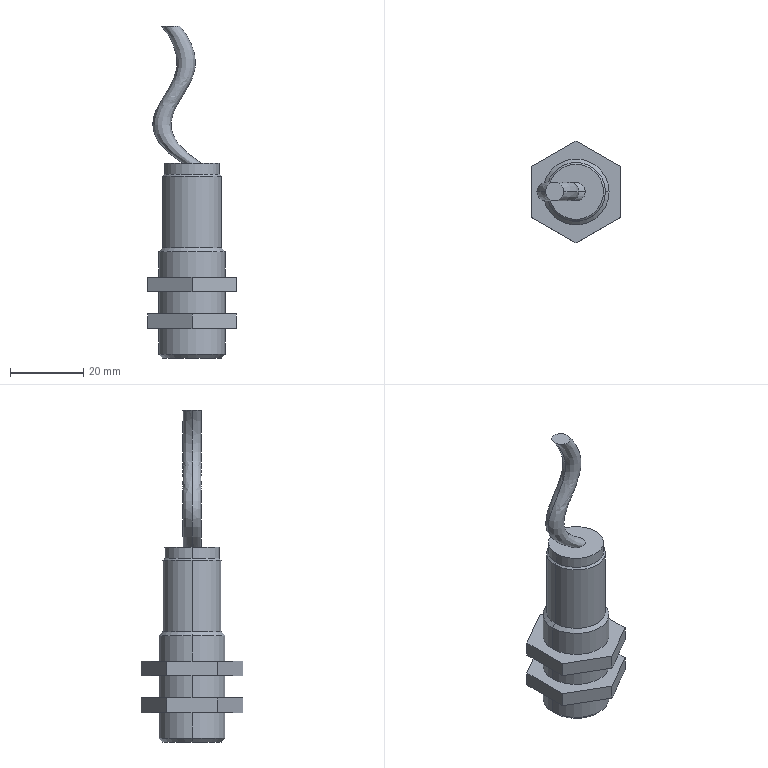Part | SolidWorks | features ICE 3, Chamfer 2, Extrusion 1, MirrorPattern 1, Sweep 1 | 1 solid | 37 faces | box 24 x 27.713 x 90.43 mm | volume 14815 mm3 | plane 19 | cylinder 10 | cone 6 | spline 2 | commonest cylinder face diameters 18 x6 15 x2 16 x2
STEP:
#1=CARTESIAN_POINT('',(9.,0.,-7.));
#2=VERTEX_POINT('',#1);
#3=CARTESIAN_POINT('',(-9.,0.,-7.));
#4=VERTEX_POINT('',#3);
#5=CARTESIAN_POINT('',(0.,0.,-7.));
#6=DIRECTION('',(0.,0.,1.));
#7=DIRECTION('',(1.,0.,0.));
#8=AXIS2_PLACEMENT_3D('',#5,#6,#7);
#9=CIRCLE('',#8,9.);
#10=EDGE_CURVE('',#2,#4,#9,.T.);
#11=ORIENTED_EDGE('',*,*,#10,.F.);
#12=CARTESIAN_POINT('',(9.,0.,-14.));
#13=VERTEX_POINT('',#12);
#14=CARTESIAN_POINT('',(9.,0.,15.));
#15=DIRECTION('',(0.,0.,-1.));
#16=VECTOR('',#15,1000.);
#17=LINE('',#14,#16);
#18=EDGE_CURVE('',#2,#13,#17,.T.);
#19=ORIENTED_EDGE('',*,*,#18,.T.);
#20=CARTESIAN_POINT('',(-9.,0.,-14.));
#21=VERTEX_POINT('',#20);
#22=CARTESIAN_POINT('',(0.,0.,-14.));
#23=DIRECTION('',(0.,0.,1.));
#24=DIRECTION('',(1.,0.,0.));
#25=AXIS2_PLACEMENT_3D('',#22,#23,#24);
#26=CIRCLE('',#25,9.);
#27=EDGE_CURVE('',#13,#21,#26,.T.);
#28=ORIENTED_EDGE('',*,*,#27,.T.);
#29=CARTESIAN_POINT('',(-9.,0.,15.));
#30=DIRECTION('',(0.,0.,-1.));
#31=VECTOR('',#30,1000.);
#32=LINE('',#29,#31);
#33=EDGE_CURVE('',#4,#21,#32,.T.);
#34=ORIENTED_EDGE('',*,*,#33,.F.);
#35=EDGE_LOOP('',(#11,#19,#28,#34));
#36=FACE_OUTER_BOUND('',#35,.T.);
#37=CARTESIAN_POINT('',(0.,0.,15.));
#38=DIRECTION('',(0.,0.,-1.));
#39=DIRECTION('',(-1.,0.,0.));
#40=AXIS2_PLACEMENT_3D('',#37,#38,#39);
#41=CYLINDRICAL_SURFACE('',#40,9.);
#42=ADVANCED_FACE('',(#36),#41,.T.);
#43=CARTESIAN_POINT('',(-8.,0.,-15.));
#44=VERTEX_POINT('',#43);
#45=CARTESIAN_POINT('',(8.,0.,-15.));
#46=VERTEX_POINT('',#45);
#47=CARTESIAN_POINT('',(0.,0.,-15.));
#48=DIRECTION('',(0.,0.,-1.));
#49=DIRECTION('',(1.,0.,0.));
#50=AXIS2_PLACEMENT_3D('',#47,#48,#49);
#51=CIRCLE('',#50,8.);
#52=EDGE_CURVE('',#44,#46,#51,.T.);
#53=ORIENTED_EDGE('',*,*,#52,.F.);
#54=CARTESIAN_POINT('',(-9.,0.,-14.));
#55=DIRECTION('',(-0.7071,0.,0.7071));
#56=VECTOR('',#55,1000.);
#57=LINE('',#54,#56);
#58=EDGE_CURVE('',#44,#21,#57,.T.);
#59=ORIENTED_EDGE('',*,*,#58,.T.);
#60=ORIENTED_EDGE('',*,*,#27,.F.);
#61=CARTESIAN_POINT('',(9.,0.,-14.));
#62=DIRECTION('',(0.7071,0.,0.7071));
#63=VECTOR('',#62,1000.);
#64=LINE('',#61,#63);
#65=EDGE_CURVE('',#46,#13,#64,.T.);
#66=ORIENTED_EDGE('',*,*,#65,.F.);
#67=EDGE_LOOP('',(#53,#59,#60,#66));
#68=FACE_OUTER_BOUND('',#67,.T.);
#69=CARTESIAN_POINT('',(0.,0.,-14.));
#70=DIRECTION('',(0.,0.,1.));
#71=DIRECTION('',(1.,0.,0.));
#72=AXIS2_PLACEMENT_3D('',#69,#70,#71);
#73=CONICAL_SURFACE('',#72,9.,0.7854);
#74=ADVANCED_FACE('',(#68),#73,.T.);
#75=CARTESIAN_POINT('',(2.5,0.,38.));
#76=VERTEX_POINT('',#75);
#77=CARTESIAN_POINT('',(-2.5,0.,38.));
#78=VERTEX_POINT('',#77);
#79=CARTESIAN_POINT('',(0.,0.,38.));
#80=DIRECTION('',(0.,0.,1.));
#81=DIRECTION('',(1.,0.,0.));
#82=AXIS2_PLACEMENT_3D('',#79,#80,#81);
#83=CIRCLE('',#82,2.5);
#84=EDGE_CURVE('',#76,#78,#83,.T.);
#85=ORIENTED_EDGE('',*,*,#84,.T.);
#86=CARTESIAN_POINT('',(-8.322,0.,75.43));
#87=VERTEX_POINT('',#86);
#88=CARTESIAN_POINT('',(-2.5,0.,38.));
#89=CARTESIAN_POINT('',(-3.213,0.,38.463));
#90=CARTESIAN_POINT('',(-4.676,0.,39.476));
#91=CARTESIAN_POINT('',(-6.384,0.,40.858));
#92=CARTESIAN_POINT('',(-7.796,0.,42.216));
#93=CARTESIAN_POINT('',(-8.893,0.,43.524));
#94=CARTESIAN_POINT('',(-9.71,0.,44.794));
#95=CARTESIAN_POINT('',(-10.269,0.,46.027));
#96=CARTESIAN_POINT('',(-10.595,0.,47.228));
#97=CARTESIAN_POINT('',(-10.829,0.,49.572));
#98=CARTESIAN_POINT('',(-9.799,0.,52.906));
#99=CARTESIAN_POINT('',(-7.043,0.,57.206));
#100=CARTESIAN_POINT('',(-4.896,0.,60.875));
#101=CARTESIAN_POINT('',(-4.052,0.,63.985));
#102=CARTESIAN_POINT('',(-4.046,0.,66.435));
#103=CARTESIAN_POINT('',(-4.646,0.,69.312));
#104=CARTESIAN_POINT('',(-6.067,0.,72.499));
#105=CARTESIAN_POINT('',(-7.5,0.,74.501));
#106=CARTESIAN_POINT('',(-8.322,0.,75.43));
#107=B_SPLINE_CURVE_WITH_KNOTS('',3,(#88,#89,#90,#91,#92,#93,#94,#95,#96,#97,#98,#99,#100,#101,#102,#103,#104,#105,#106),.UNSPECIFIED.,.F.,.F.,(4,1,1,1,1,1,1,1,1,1,1,1,1,1,1,1,4),(0.,0.03125,0.0625,0.09375,0.125,0.1562,0.1875,0.2187,0.25,0.375,0.5,0.625,0.6875,0.75,0.8125,0.9062,1.),.UNSPECIFIED.);
#108=EDGE_CURVE('',#78,#87,#107,.T.);
#109=ORIENTED_EDGE('',*,*,#108,.T.);
#110=CARTESIAN_POINT('',(-3.322,0.,75.43));
#111=VERTEX_POINT('',#110);
#112=CARTESIAN_POINT('',(-5.822,0.,75.43));
#113=DIRECTION('',(0.,0.,1.));
#114=DIRECTION('',(1.,0.,0.));
#115=AXIS2_PLACEMENT_3D('',#112,#113,#114);
#116=CIRCLE('',#115,2.5);
#117=EDGE_CURVE('',#111,#87,#116,.T.);
#118=ORIENTED_EDGE('',*,*,#117,.F.);
#119=CARTESIAN_POINT('',(2.5,0.,38.));
#120=CARTESIAN_POINT('',(1.787,0.,38.463));
#121=CARTESIAN_POINT('',(0.3238,0.,39.476));
#122=CARTESIAN_POINT('',(-1.384,0.,40.858));
#123=CARTESIAN_POINT('',(-2.796,0.,42.216));
#124=CARTESIAN_POINT('',(-3.893,0.,43.524));
#125=CARTESIAN_POINT('',(-4.71,0.,44.794));
#126=CARTESIAN_POINT('',(-5.269,0.,46.027));
#127=CARTESIAN_POINT('',(-5.595,0.,47.228));
#128=CARTESIAN_POINT('',(-5.829,0.,49.572));
#129=CARTESIAN_POINT('',(-4.799,0.,52.906));
#130=CARTESIAN_POINT('',(-2.043,0.,57.206));
#131=CARTESIAN_POINT('',(0.1038,0.,60.875));
#132=CARTESIAN_POINT('',(0.9476,0.,63.985));
#133=CARTESIAN_POINT('',(0.9535,0.,66.435));
#134=CARTESIAN_POINT('',(0.3536,0.,69.312));
#135=CARTESIAN_POINT('',(-1.067,0.,72.499));
#136=CARTESIAN_POINT('',(-2.5,0.,74.501));
#137=CARTESIAN_POINT('',(-3.322,0.,75.43));
#138=B_SPLINE_CURVE_WITH_KNOTS('',3,(#119,#120,#121,#122,#123,#124,#125,#126,#127,#128,#129,#130,#131,#132,#133,#134,#135,#136,#137),.UNSPECIFIED.,.F.,.F.,(4,1,1,1,1,1,1,1,1,1,1,1,1,1,1,1,4),(0.,0.03125,0.0625,0.09375,0.125,0.1562,0.1875,0.2187,0.25,0.375,0.5,0.625,0.6875,0.75,0.8125,0.9062,1.),.UNSPECIFIED.);
#139=EDGE_CURVE('',#76,#111,#138,.T.);
#140=ORIENTED_EDGE('',*,*,#139,.F.);
#141=EDGE_LOOP('',(#85,#109,#118,#140));
#142=FACE_OUTER_BOUND('',#141,.T.);
#143=CARTESIAN_POINT('',(2.5,0.,38.));
#144=CARTESIAN_POINT('',(1.787,0.,38.463));
#145=CARTESIAN_POINT('',(0.3238,0.,39.476));
#146=CARTESIAN_POINT('',(-1.384,0.,40.858));
#147=CARTESIAN_POINT('',(-2.796,0.,42.216));
#148=CARTESIAN_POINT('',(-3.893,0.,43.524));
#149=CARTESIAN_POINT('',(-4.71,0.,44.794));
#150=CARTESIAN_POINT('',(-5.269,0.,46.027));
#151=CARTESIAN_POINT('',(-5.595,0.,47.228));
#152=CARTESIAN_POINT('',(-5.829,0.,49.572));
#153=CARTESIAN_POINT('',(-4.799,0.,52.906));
#154=CARTESIAN_POINT('',(-2.043,0.,57.206));
#155=CARTESIAN_POINT('',(0.1038,0.,60.875));
#156=CARTESIAN_POINT('',(0.9476,0.,63.985));
#157=CARTESIAN_POINT('',(0.9535,0.,66.435));
#158=CARTESIAN_POINT('',(0.3536,0.,69.312));
#159=CARTESIAN_POINT('',(-1.067,0.,72.499));
#160=CARTESIAN_POINT('',(-2.5,0.,74.501));
#161=CARTESIAN_POINT('',(-3.322,0.,75.43));
#162=CARTESIAN_POINT('',(2.5,5.,38.));
#163=CARTESIAN_POINT('',(1.787,5.,38.463));
#164=CARTESIAN_POINT('',(0.3238,5.,39.476));
#165=CARTESIAN_POINT('',(-1.384,5.,40.858));
#166=CARTESIAN_POINT('',(-2.796,5.,42.216));
#167=CARTESIAN_POINT('',(-3.893,5.,43.524));
#168=CARTESIAN_POINT('',(-4.71,5.,44.794));
#169=CARTESIAN_POINT('',(-5.269,5.,46.027));
#170=CARTESIAN_POINT('',(-5.595,5.,47.228));
#171=CARTESIAN_POINT('',(-5.829,5.,49.572));
#172=CARTESIAN_POINT('',(-4.799,5.,52.906));
#173=CARTESIAN_POINT('',(-2.043,5.,57.206));
#174=CARTESIAN_POINT('',(0.1038,5.,60.875));
#175=CARTESIAN_POINT('',(0.9476,5.,63.985));
#176=CARTESIAN_POINT('',(0.9535,5.,66.435));
#177=CARTESIAN_POINT('',(0.3536,5.,69.312));
#178=CARTESIAN_POINT('',(-1.067,5.,72.499));
#179=CARTESIAN_POINT('',(-2.5,5.,74.501));
#180=CARTESIAN_POINT('',(-3.322,5.,75.43));
#181=CARTESIAN_POINT('',(-2.5,5.,38.));
#182=CARTESIAN_POINT('',(-3.213,5.,38.463));
#183=CARTESIAN_POINT('',(-4.676,5.,39.476));
#184=CARTESIAN_POINT('',(-6.384,5.,40.858));
#185=CARTESIAN_POINT('',(-7.796,5.,42.216));
#186=CARTESIAN_POINT('',(-8.893,5.,43.524));
#187=CARTESIAN_POINT('',(-9.71,5.,44.794));
#188=CARTESIAN_POINT('',(-10.269,5.,46.027));
#189=CARTESIAN_POINT('',(-10.595,5.,47.228));
#190=CARTESIAN_POINT('',(-10.829,5.,49.572));
#191=CARTESIAN_POINT('',(-9.799,5.,52.906));
#192=CARTESIAN_POINT('',(-7.043,5.,57.206));
#193=CARTESIAN_POINT('',(-4.896,5.,60.875));
#194=CARTESIAN_POINT('',(-4.052,5.,63.985));
#195=CARTESIAN_POINT('',(-4.046,5.,66.435));
#196=CARTESIAN_POINT('',(-4.646,5.,69.312));
#197=CARTESIAN_POINT('',(-6.067,5.,72.499));
#198=CARTESIAN_POINT('',(-7.5,5.,74.501));
#199=CARTESIAN_POINT('',(-8.322,5.,75.43));
#200=CARTESIAN_POINT('',(-2.5,0.,38.));
#201=CARTESIAN_POINT('',(-3.213,0.,38.463));
#202=CARTESIAN_POINT('',(-4.676,0.,39.476));
#203=CARTESIAN_POINT('',(-6.384,0.,40.858));
#204=CARTESIAN_POINT('',(-7.796,0.,42.216));
#205=CARTESIAN_POINT('',(-8.893,0.,43.524));
#206=CARTESIAN_POINT('',(-9.71,0.,44.794));
#207=CARTESIAN_POINT('',(-10.269,0.,46.027));
#208=CARTESIAN_POINT('',(-10.595,0.,47.228));
#209=CARTESIAN_POINT('',(-10.829,0.,49.572));
#210=CARTESIAN_POINT('',(-9.799,0.,52.906));
#211=CARTESIAN_POINT('',(-7.043,0.,57.206));
#212=CARTESIAN_POINT('',(-4.896,0.,60.875));
#213=CARTESIAN_POINT('',(-4.052,0.,63.985));
#214=CARTESIAN_POINT('',(-4.046,0.,66.435));
#215=CARTESIAN_POINT('',(-4.646,0.,69.312));
#216=CARTESIAN_POINT('',(-6.067,0.,72.499));
#217=CARTESIAN_POINT('',(-7.5,0.,74.501));
#218=CARTESIAN_POINT('',(-8.322,0.,75.43));
#219=CARTESIAN_POINT('',(-2.5,-5.,38.));
#220=CARTESIAN_POINT('',(-3.213,-5.,38.463));
#221=CARTESIAN_POINT('',(-4.676,-5.,39.476));
#222=CARTESIAN_POINT('',(-6.384,-5.,40.858));
#223=CARTESIAN_POINT('',(-7.796,-5.,42.216));
#224=CARTESIAN_POINT('',(-8.893,-5.,43.524));
#225=CARTESIAN_POINT('',(-9.71,-5.,44.794));
#226=CARTESIAN_POINT('',(-10.269,-5.,46.027));
#227=CARTESIAN_POINT('',(-10.595,-5.,47.228));
#228=CARTESIAN_POINT('',(-10.829,-5.,49.572));
#229=CARTESIAN_POINT('',(-9.799,-5.,52.906));
#230=CARTESIAN_POINT('',(-7.043,-5.,57.206));
#231=CARTESIAN_POINT('',(-4.896,-5.,60.875));
#232=CARTESIAN_POINT('',(-4.052,-5.,63.985));
#233=CARTESIAN_POINT('',(-4.046,-5.,66.435));
#234=CARTESIAN_POINT('',(-4.646,-5.,69.312));
#235=CARTESIAN_POINT('',(-6.067,-5.,72.499));
#236=CARTESIAN_POINT('',(-7.5,-5.,74.501));
#237=CARTESIAN_POINT('',(-8.322,-5.,75.43));
#238=CARTESIAN_POINT('',(2.5,-5.,38.));
#239=CARTESIAN_POINT('',(1.787,-5.,38.463));
#240=CARTESIAN_POINT('',(0.3238,-5.,39.476));
#241=CARTESIAN_POINT('',(-1.384,-5.,40.858));
#242=CARTESIAN_POINT('',(-2.796,-5.,42.216));
#243=CARTESIAN_POINT('',(-3.893,-5.,43.524));
#244=CARTESIAN_POINT('',(-4.71,-5.,44.794));
#245=CARTESIAN_POINT('',(-5.269,-5.,46.027));
#246=CARTESIAN_POINT('',(-5.595,-5.,47.228));
#247=CARTESIAN_POINT('',(-5.829,-5.,49.572));
#248=CARTESIAN_POINT('',(-4.799,-5.,52.906));
#249=CARTESIAN_POINT('',(-2.043,-5.,57.206));
#250=CARTESIAN_POINT('',(0.1038,-5.,60.875));
#251=CARTESIAN_POINT('',(0.9476,-5.,63.985));
#252=CARTESIAN_POINT('',(0.9535,-5.,66.435));
#253=CARTESIAN_POINT('',(0.3536,-5.,69.312));
#254=CARTESIAN_POINT('',(-1.067,-5.,72.499));
#255=CARTESIAN_POINT('',(-2.5,-5.,74.501));
#256=CARTESIAN_POINT('',(-3.322,-5.,75.43));
#257=CARTESIAN_POINT('',(2.5,0.,38.));
#258=CARTESIAN_POINT('',(1.787,0.,38.463));
#259=CARTESIAN_POINT('',(0.3238,0.,39.476));
#260=CARTESIAN_POINT('',(-1.384,0.,40.858));
#261=CARTESIAN_POINT('',(-2.796,0.,42.216));
#262=CARTESIAN_POINT('',(-3.893,0.,43.524));
#263=CARTESIAN_POINT('',(-4.71,0.,44.794));
#264=CARTESIAN_POINT('',(-5.269,0.,46.027));
#265=CARTESIAN_POINT('',(-5.595,0.,47.228));
#266=CARTESIAN_POINT('',(-5.829,0.,49.572));
#267=CARTESIAN_POINT('',(-4.799,0.,52.906));
#268=CARTESIAN_POINT('',(-2.043,0.,57.206));
#269=CARTESIAN_POINT('',(0.1038,0.,60.875));
#270=CARTESIAN_POINT('',(0.9476,0.,63.985));
#271=CARTESIAN_POINT('',(0.9535,0.,66.435));
#272=CARTESIAN_POINT('',(0.3536,0.,69.312));
#273=CARTESIAN_POINT('',(-1.067,0.,72.499));
#274=CARTESIAN_POINT('',(-2.5,0.,74.501));
#275=CARTESIAN_POINT('',(-3.322,0.,75.43));
#276=(BOUNDED_SURFACE()B_SPLINE_SURFACE(3,3,((#143,#144,#145,#146,#147,#148,#149,#150,#151,#152,#153,#154,#155,#156,#157,#158,#159,#160,#161),(#162,#163,#164,#165,#166,#167,#168,#169,#170,#171,#172,#173,#174,#175,#176,#177,#178,#179,#180),(#181,#182,#183,#184,#185,#186,#187,#188,#189,#190,#191,#192,#193,#194,#195,#196,#197,#198,#199),(#200,#201,#202,#203,#204,#205,#206,#207,#208,#209,#210,#211,#212,#213,#214,#215,#216,#217,#218),(#219,#220,#221,#222,#223,#224,#225,#226,#227,#228,#229,#230,#231,#232,#233,#234,#235,#236,#237),(#238,#239,#240,#241,#242,#243,#244,#245,#246,#247,#248,#249,#250,#251,#252,#253,#254,#255,#256),(#257,#258,#259,#260,#261,#262,#263,#264,#265,#266,#267,#268,#269,#270,#271,#272,#273,#274,#275)),.UNSPECIFIED.,.T.,.F.,.T.)B_SPLINE_SURFACE_WITH_KNOTS((4,3,4),(4,1,1,1,1,1,1,1,1,1,1,1,1,1,1,1,4),(0.,0.5,1.),(0.,0.03125,0.0625,0.09375,0.125,0.1562,0.1875,0.2187,0.25,0.375,0.5,0.625,0.6875,0.75,0.8125,0.9062,1.),.UNSPECIFIED.)GEOMETRIC_REPRESENTATION_ITEM()RATIONAL_B_SPLINE_SURFACE(((1.,1.,1.,1.,1.,1.,1.,1.,1.,1.,1.,1.,1.,1.,1.,1.,1.,1.,1.),(0.3333,0.3333,0.3333,0.3333,0.3333,0.3333,0.3333,0.3333,0.3333,0.3333,0.3333,0.3333,0.3333,0.3333,0.3333,0.3333,0.3333,0.3333,0.3333),(0.3333,0.3333,0.3333,0.3333,0.3333,0.3333,0.3333,0.3333,0.3333,0.3333,0.3333,0.3333,0.3333,0.3333,0.3333,0.3333,0.3333,0.3333,0.3333),(1.,1.,1.,1.,1.,1.,1.,1.,1.,1.,1.,1.,1.,1.,1.,1.,1.,1.,1.),(0.3333,0.3333,0.3333,0.3333,0.3333,0.3333,0.3333,0.3333,0.3333,0.3333,0.3333,0.3333,0.3333,0.3333,0.3333,0.3333,0.3333,0.3333,0.3333),(0.3333,0.3333,0.3333,0.3333,0.3333,0.3333,0.3333,0.3333,0.3333,0.3333,0.3333,0.3333,0.3333,0.3333,0.3333,0.3333,0.3333,0.3333,0.3333),(1.,1.,1.,1.,1.,1.,1.,1.,1.,1.,1.,1.,1.,1.,1.,1.,1.,1.,1.)))REPRESENTATION_ITEM('')SURFACE());
#277=ADVANCED_FACE('',(#142),#276,.T.);
#278=CARTESIAN_POINT('',(7.5,0.,35.));
#279=VERTEX_POINT('',#278);
#280=CARTESIAN_POINT('',(-7.5,0.,35.));
#281=VERTEX_POINT('',#280);
#282=CARTESIAN_POINT('',(0.,0.,35.));
#283=DIRECTION('',(0.,0.,1.));
#284=DIRECTION('',(1.,0.,0.));
#285=AXIS2_PLACEMENT_3D('',#282,#283,#284);
#286=CIRCLE('',#285,7.5);
#287=EDGE_CURVE('',#279,#281,#286,.T.);
#288=ORIENTED_EDGE('',*,*,#287,.F.);
#289=CARTESIAN_POINT('',(8.,0.,34.5));
#290=VERTEX_POINT('',#289);
#291=CARTESIAN_POINT('',(7.5,0.,35.));
#292=DIRECTION('',(0.7071,0.,-0.7071));
#293=VECTOR('',#292,1000.);
#294=LINE('',#291,#293);
#295=EDGE_CURVE('',#279,#290,#294,.T.);
#296=ORIENTED_EDGE('',*,*,#295,.T.);
#297=CARTESIAN_POINT('',(-8.,0.,34.5));
#298=VERTEX_POINT('',#297);
#299=CARTESIAN_POINT('',(0.,0.,34.5));
#300=DIRECTION('',(0.,0.,-1.));
#301=DIRECTION('',(1.,0.,0.));
#302=AXIS2_PLACEMENT_3D('',#299,#300,#301);
#303=CIRCLE('',#302,8.);
#304=EDGE_CURVE('',#298,#290,#303,.T.);
#305=ORIENTED_EDGE('',*,*,#304,.F.);
#306=CARTESIAN_POINT('',(-7.5,0.,35.));
#307=DIRECTION('',(-0.7071,0.,-0.7071));
#308=VECTOR('',#307,1000.);
#309=LINE('',#306,#308);
#310=EDGE_CURVE('',#281,#298,#309,.T.);
#311=ORIENTED_EDGE('',*,*,#310,.F.);
#312=EDGE_LOOP('',(#288,#296,#305,#311));
#313=FACE_OUTER_BOUND('',#312,.T.);
#314=CARTESIAN_POINT('',(0.,0.,35.));
#315=DIRECTION('',(0.,0.,-1.));
#316=DIRECTION('',(-1.,0.,0.));
#317=AXIS2_PLACEMENT_3D('',#314,#315,#316);
#318=CONICAL_SURFACE('',#317,7.5,0.7854);
#319=ADVANCED_FACE('',(#313),#318,.T.);
#320=CARTESIAN_POINT('',(7.5,0.,38.));
#321=VERTEX_POINT('',#320);
#322=CARTESIAN_POINT('',(-7.5,0.,38.));
#323=VERTEX_POINT('',#322);
#324=CARTESIAN_POINT('',(0.,0.,38.));
#325=DIRECTION('',(0.,0.,1.));
#326=DIRECTION('',(1.,0.,0.));
#327=AXIS2_PLACEMENT_3D('',#324,#325,#326);
#328=CIRCLE('',#327,7.5);
#329=EDGE_CURVE('',#321,#323,#328,.T.);
#330=ORIENTED_EDGE('',*,*,#329,.F.);
#331=CARTESIAN_POINT('',(7.5,0.,38.));
#332=DIRECTION('',(0.,0.,-1.));
#333=VECTOR('',#332,1000.);
#334=LINE('',#331,#333);
#335=EDGE_CURVE('',#321,#279,#334,.T.);
#336=ORIENTED_EDGE('',*,*,#335,.T.);
#337=ORIENTED_EDGE('',*,*,#287,.T.);
#338=CARTESIAN_POINT('',(-7.5,0.,38.));
#339=DIRECTION('',(0.,0.,-1.));
#340=VECTOR('',#339,1000.);
#341=LINE('',#338,#340);
#342=EDGE_CURVE('',#323,#281,#341,.T.);
#343=ORIENTED_EDGE('',*,*,#342,.F.);
#344=EDGE_LOOP('',(#330,#336,#337,#343));
#345=FACE_OUTER_BOUND('',#344,.T.);
#346=CARTESIAN_POINT('',(0.,0.,38.));
#347=DIRECTION('',(0.,0.,-1.));
#348=DIRECTION('',(-1.,0.,0.));
#349=AXIS2_PLACEMENT_3D('',#346,#347,#348);
#350=CYLINDRICAL_SURFACE('',#349,7.5);
#351=ADVANCED_FACE('',(#345),#350,.T.);
#352=ORIENTED_EDGE('',*,*,#304,.T.);
#353=CARTESIAN_POINT('',(8.,0.,15.));
#354=VERTEX_POINT('',#353);
#355=CARTESIAN_POINT('',(8.,0.,35.));
#356=DIRECTION('',(0.,0.,-1.));
#357=VECTOR('',#356,1000.);
#358=LINE('',#355,#357);
#359=EDGE_CURVE('',#290,#354,#358,.T.);
#360=ORIENTED_EDGE('',*,*,#359,.T.);
#361=CARTESIAN_POINT('',(-8.,0.,15.));
#362=VERTEX_POINT('',#361);
#363=CARTESIAN_POINT('',(0.,0.,15.));
#364=DIRECTION('',(0.,0.,1.));
#365=DIRECTION('',(1.,0.,0.));
#366=AXIS2_PLACEMENT_3D('',#363,#364,#365);
#367=CIRCLE('',#366,8.);
#368=EDGE_CURVE('',#354,#362,#367,.T.);
#369=ORIENTED_EDGE('',*,*,#368,.T.);
#370=CARTESIAN_POINT('',(-8.,0.,35.));
#371=DIRECTION('',(0.,0.,-1.));
#372=VECTOR('',#371,1000.);
#373=LINE('',#370,#372);
#374=EDGE_CURVE('',#298,#362,#373,.T.);
#375=ORIENTED_EDGE('',*,*,#374,.F.);
#376=EDGE_LOOP('',(#352,#360,#369,#375));
#377=FACE_OUTER_BOUND('',#376,.T.);
#378=CARTESIAN_POINT('',(0.,0.,35.));
#379=DIRECTION('',(0.,0.,-1.));
#380=DIRECTION('',(-1.,0.,0.));
#381=AXIS2_PLACEMENT_3D('',#378,#379,#380);
#382=CYLINDRICAL_SURFACE('',#381,8.);
#383=ADVANCED_FACE('',(#377),#382,.T.);
#384=ORIENTED_EDGE('',*,*,#368,.F.);
#385=CARTESIAN_POINT('',(9.,0.,14.));
#386=VERTEX_POINT('',#385);
#387=CARTESIAN_POINT('',(8.,0.,15.));
#388=DIRECTION('',(0.7071,0.,-0.7071));
#389=VECTOR('',#388,1000.);
#390=LINE('',#387,#389);
#391=EDGE_CURVE('',#354,#386,#390,.T.);
#392=ORIENTED_EDGE('',*,*,#391,.T.);
#393=CARTESIAN_POINT('',(-9.,0.,14.));
#394=VERTEX_POINT('',#393);
#395=CARTESIAN_POINT('',(0.,0.,14.));
#396=DIRECTION('',(0.,0.,-1.));
#397=DIRECTION('',(1.,0.,0.));
#398=AXIS2_PLACEMENT_3D('',#395,#396,#397);
#399=CIRCLE('',#398,9.);
#400=EDGE_CURVE('',#394,#386,#399,.T.);
#401=ORIENTED_EDGE('',*,*,#400,.F.);
#402=CARTESIAN_POINT('',(-8.,0.,15.));
#403=DIRECTION('',(-0.7071,0.,-0.7071));
#404=VECTOR('',#403,1000.);
#405=LINE('',#402,#404);
#406=EDGE_CURVE('',#362,#394,#405,.T.);
#407=ORIENTED_EDGE('',*,*,#406,.F.);
#408=EDGE_LOOP('',(#384,#392,#401,#407));
#409=FACE_OUTER_BOUND('',#408,.T.);
#410=CARTESIAN_POINT('',(0.,0.,15.));
#411=DIRECTION('',(0.,0.,-1.));
#412=DIRECTION('',(-1.,0.,0.));
#413=AXIS2_PLACEMENT_3D('',#410,#411,#412);
#414=CONICAL_SURFACE('',#413,8.,0.7854);
#415=ADVANCED_FACE('',(#409),#414,.T.);
#416=ORIENTED_EDGE('',*,*,#400,.T.);
#417=CARTESIAN_POINT('',(9.,0.,7.));
#418=VERTEX_POINT('',#417);
#419=CARTESIAN_POINT('',(9.,0.,15.));
#420=DIRECTION('',(0.,0.,-1.));
#421=VECTOR('',#420,1000.);
#422=LINE('',#419,#421);
#423=EDGE_CURVE('',#386,#418,#422,.T.);
#424=ORIENTED_EDGE('',*,*,#423,.T.);
#425=CARTESIAN_POINT('',(-9.,0.,7.));
#426=VERTEX_POINT('',#425);
#427=CARTESIAN_POINT('',(0.,0.,7.));
#428=DIRECTION('',(0.,0.,1.));
#429=DIRECTION('',(1.,0.,0.));
#430=AXIS2_PLACEMENT_3D('',#427,#428,#429);
#431=CIRCLE('',#430,9.);
#432=EDGE_CURVE('',#418,#426,#431,.T.);
#433=ORIENTED_EDGE('',*,*,#432,.T.);
#434=CARTESIAN_POINT('',(-9.,0.,15.));
#435=DIRECTION('',(0.,0.,-1.));
#436=VECTOR('',#435,1000.);
#437=LINE('',#434,#436);
#438=EDGE_CURVE('',#394,#426,#437,.T.);
#439=ORIENTED_EDGE('',*,*,#438,.F.);
#440=EDGE_LOOP('',(#416,#424,#433,#439));
#441=FACE_OUTER_BOUND('',#440,.T.);
#442=CARTESIAN_POINT('',(0.,0.,15.));
#443=DIRECTION('',(0.,0.,-1.));
#444=DIRECTION('',(-1.,0.,0.));
#445=AXIS2_PLACEMENT_3D('',#442,#443,#444);
#446=CYLINDRICAL_SURFACE('',#445,9.);
#447=ADVANCED_FACE('',(#441),#446,.T.);
#448=CARTESIAN_POINT('',(9.,0.,3.));
#449=VERTEX_POINT('',#448);
#450=CARTESIAN_POINT('',(-9.,0.,3.));
#451=VERTEX_POINT('',#450);
#452=CARTESIAN_POINT('',(0.,0.,3.));
#453=DIRECTION('',(0.,0.,1.));
#454=DIRECTION('',(1.,0.,0.));
#455=AXIS2_PLACEMENT_3D('',#452,#453,#454);
#456=CIRCLE('',#455,9.);
#457=EDGE_CURVE('',#449,#451,#456,.T.);
#458=ORIENTED_EDGE('',*,*,#457,.F.);
#459=CARTESIAN_POINT('',(9.,0.,-3.));
#460=VERTEX_POINT('',#459);
#461=CARTESIAN_POINT('',(9.,0.,15.));
#462=DIRECTION('',(0.,0.,-1.));
#463=VECTOR('',#462,1000.);
#464=LINE('',#461,#463);
#465=EDGE_CURVE('',#449,#460,#464,.T.);
#466=ORIENTED_EDGE('',*,*,#465,.T.);
#467=CARTESIAN_POINT('',(-9.,0.,-3.));
#468=VERTEX_POINT('',#467);
#469=CARTESIAN_POINT('',(0.,0.,-3.));
#470=DIRECTION('',(0.,0.,-1.));
#471=DIRECTION('',(-1.,0.,0.));
#472=AXIS2_PLACEMENT_3D('',#469,#470,#471);
#473=CIRCLE('',#472,9.);
#474=EDGE_CURVE('',#468,#460,#473,.T.);
#475=ORIENTED_EDGE('',*,*,#474,.F.);
#476=CARTESIAN_POINT('',(-9.,0.,15.));
#477=DIRECTION('',(0.,0.,-1.));
#478=VECTOR('',#477,1000.);
#479=LINE('',#476,#478);
#480=EDGE_CURVE('',#451,#468,#479,.T.);
#481=ORIENTED_EDGE('',*,*,#480,.F.);
#482=EDGE_LOOP('',(#458,#466,#475,#481));
#483=FACE_OUTER_BOUND('',#482,.T.);
#484=CARTESIAN_POINT('',(0.,0.,15.));
#485=DIRECTION('',(0.,0.,-1.));
#486=DIRECTION('',(-1.,0.,0.));
#487=AXIS2_PLACEMENT_3D('',#484,#485,#486);
#488=CYLINDRICAL_SURFACE('',#487,9.);
#489=ADVANCED_FACE('',(#483),#488,.T.);
#490=ORIENTED_EDGE('',*,*,#465,.F.);
#491=CARTESIAN_POINT('',(0.,0.,3.));
#492=DIRECTION('',(0.,0.,1.));
#493=DIRECTION('',(1.,0.,0.));
#494=AXIS2_PLACEMENT_3D('',#491,#492,#493);
#495=CIRCLE('',#494,9.);
#496=EDGE_CURVE('',#451,#449,#495,.T.);
#497=ORIENTED_EDGE('',*,*,#496,.F.);
#498=ORIENTED_EDGE('',*,*,#480,.T.);
#499=CARTESIAN_POINT('',(0.,0.,-3.));
#500=DIRECTION('',(0.,0.,-1.));
#501=DIRECTION('',(-1.,0.,0.));
#502=AXIS2_PLACEMENT_3D('',#499,#500,#501);
#503=CIRCLE('',#502,9.);
#504=EDGE_CURVE('',#460,#468,#503,.T.);
#505=ORIENTED_EDGE('',*,*,#504,.F.);
#506=EDGE_LOOP('',(#490,#497,#498,#505));
#507=FACE_OUTER_BOUND('',#506,.T.);
#508=CARTESIAN_POINT('',(0.,0.,15.));
#509=DIRECTION('',(0.,0.,-1.));
#510=DIRECTION('',(-1.,0.,0.));
#511=AXIS2_PLACEMENT_3D('',#508,#509,#510);
#512=CYLINDRICAL_SURFACE('',#511,9.);
#513=ADVANCED_FACE('',(#507),#512,.T.);
#514=ORIENTED_EDGE('',*,*,#423,.F.);
#515=CARTESIAN_POINT('',(0.,0.,14.));
#516=DIRECTION('',(0.,0.,-1.));
#517=DIRECTION('',(1.,0.,0.));
#518=AXIS2_PLACEMENT_3D('',#515,#516,#517);
#519=CIRCLE('',#518,9.);
#520=EDGE_CURVE('',#386,#394,#519,.T.);
#521=ORIENTED_EDGE('',*,*,#520,.T.);
#522=ORIENTED_EDGE('',*,*,#438,.T.);
#523=CARTESIAN_POINT('',(0.,0.,7.));
#524=DIRECTION('',(0.,0.,1.));
#525=DIRECTION('',(1.,0.,0.));
#526=AXIS2_PLACEMENT_3D('',#523,#524,#525);
#527=CIRCLE('',#526,9.);
#528=EDGE_CURVE('',#426,#418,#527,.T.);
#529=ORIENTED_EDGE('',*,*,#528,.T.);
#530=EDGE_LOOP('',(#514,#521,#522,#529));
#531=FACE_OUTER_BOUND('',#530,.T.);
#532=CARTESIAN_POINT('',(0.,0.,15.));
#533=DIRECTION('',(0.,0.,-1.));
#534=DIRECTION('',(-1.,0.,0.));
#535=AXIS2_PLACEMENT_3D('',#532,#533,#534);
#536=CYLINDRICAL_SURFACE('',#535,9.);
#537=ADVANCED_FACE('',(#531),#536,.T.);
#538=ORIENTED_EDGE('',*,*,#391,.F.);
#539=CARTESIAN_POINT('',(0.,0.,15.));
#540=DIRECTION('',(0.,0.,1.));
#541=DIRECTION('',(1.,0.,0.));
#542=AXIS2_PLACEMENT_3D('',#539,#540,#541);
#543=CIRCLE('',#542,8.);
#544=EDGE_CURVE('',#362,#354,#543,.T.);
#545=ORIENTED_EDGE('',*,*,#544,.F.);
#546=ORIENTED_EDGE('',*,*,#406,.T.);
#547=ORIENTED_EDGE('',*,*,#520,.F.);
#548=EDGE_LOOP('',(#538,#545,#546,#547));
#549=FACE_OUTER_BOUND('',#548,.T.);
#550=CARTESIAN_POINT('',(0.,0.,15.));
#551=DIRECTION('',(0.,0.,-1.));
#552=DIRECTION('',(-1.,0.,0.));
#553=AXIS2_PLACEMENT_3D('',#550,#551,#552);
#554=CONICAL_SURFACE('',#553,8.,0.7854);
#555=ADVANCED_FACE('',(#549),#554,.T.);
#556=ORIENTED_EDGE('',*,*,#359,.F.);
#557=CARTESIAN_POINT('',(0.,0.,34.5));
#558=DIRECTION('',(0.,0.,-1.));
#559=DIRECTION('',(1.,0.,0.));
#560=AXIS2_PLACEMENT_3D('',#557,#558,#559);
#561=CIRCLE('',#560,8.);
#562=EDGE_CURVE('',#290,#298,#561,.T.);
#563=ORIENTED_EDGE('',*,*,#562,.T.);
#564=ORIENTED_EDGE('',*,*,#374,.T.);
#565=ORIENTED_EDGE('',*,*,#544,.T.);
#566=EDGE_LOOP('',(#556,#563,#564,#565));
#567=FACE_OUTER_BOUND('',#566,.T.);
#568=CARTESIAN_POINT('',(0.,0.,35.));
#569=DIRECTION('',(0.,0.,-1.));
#570=DIRECTION('',(-1.,0.,0.));
#571=AXIS2_PLACEMENT_3D('',#568,#569,#570);
#572=CYLINDRICAL_SURFACE('',#571,8.);
#573=ADVANCED_FACE('',(#567),#572,.T.);
#574=ORIENTED_EDGE('',*,*,#335,.F.);
#575=CARTESIAN_POINT('',(0.,0.,38.));
#576=DIRECTION('',(0.,0.,1.));
#577=DIRECTION('',(1.,0.,0.));
#578=AXIS2_PLACEMENT_3D('',#575,#576,#577);
#579=CIRCLE('',#578,7.5);
#580=EDGE_CURVE('',#323,#321,#579,.T.);
#581=ORIENTED_EDGE('',*,*,#580,.F.);
#582=ORIENTED_EDGE('',*,*,#342,.T.);
#583=CARTESIAN_POINT('',(0.,0.,35.));
#584=DIRECTION('',(0.,0.,1.));
#585=DIRECTION('',(1.,0.,0.));
#586=AXIS2_PLACEMENT_3D('',#583,#584,#585);
#587=CIRCLE('',#586,7.5);
#588=EDGE_CURVE('',#281,#279,#587,.T.);
#589=ORIENTED_EDGE('',*,*,#588,.T.);
#590=EDGE_LOOP('',(#574,#581,#582,#589));
#591=FACE_OUTER_BOUND('',#590,.T.);
#592=CARTESIAN_POINT('',(0.,0.,38.));
#593=DIRECTION('',(0.,0.,-1.));
#594=DIRECTION('',(-1.,0.,0.));
#595=AXIS2_PLACEMENT_3D('',#592,#593,#594);
#596=CYLINDRICAL_SURFACE('',#595,7.5);
#597=ADVANCED_FACE('',(#591),#596,.T.);
#598=ORIENTED_EDGE('',*,*,#84,.F.);
#599=CARTESIAN_POINT('',(0.,0.,38.));
#600=DIRECTION('',(0.,0.,1.));
#601=DIRECTION('',(1.,0.,0.));
#602=AXIS2_PLACEMENT_3D('',#599,#600,#601);
#603=CIRCLE('',#602,2.5);
#604=EDGE_CURVE('',#78,#76,#603,.T.);
#605=ORIENTED_EDGE('',*,*,#604,.F.);
#606=EDGE_LOOP('',(#598,#605));
#607=FACE_BOUND('',#606,.T.);
#608=ORIENTED_EDGE('',*,*,#580,.T.);
#609=ORIENTED_EDGE('',*,*,#329,.T.);
#610=EDGE_LOOP('',(#608,#609));
#611=FACE_OUTER_BOUND('',#610,.T.);
#612=CARTESIAN_POINT('',(0.,0.,38.));
#613=DIRECTION('',(0.,0.,1.));
#614=DIRECTION('',(1.,0.,0.));
#615=AXIS2_PLACEMENT_3D('',#612,#613,#614);
#616=PLANE('',#615);
#617=ADVANCED_FACE('',(#607,#611),#616,.T.);
#618=ORIENTED_EDGE('',*,*,#295,.F.);
#619=ORIENTED_EDGE('',*,*,#588,.F.);
#620=ORIENTED_EDGE('',*,*,#310,.T.);
#621=ORIENTED_EDGE('',*,*,#562,.F.);
#622=EDGE_LOOP('',(#618,#619,#620,#621));
#623=FACE_OUTER_BOUND('',#622,.T.);
#624=CARTESIAN_POINT('',(0.,0.,35.));
#625=DIRECTION('',(0.,0.,-1.));
#626=DIRECTION('',(-1.,0.,0.));
#627=AXIS2_PLACEMENT_3D('',#624,#625,#626);
#628=CONICAL_SURFACE('',#627,7.5,0.7854);
#629=ADVANCED_FACE('',(#623),#628,.T.);
#630=ORIENTED_EDGE('',*,*,#117,.T.);
#631=CARTESIAN_POINT('',(-5.822,0.,75.43));
#632=DIRECTION('',(0.,0.,1.));
#633=DIRECTION('',(1.,0.,0.));
#634=AXIS2_PLACEMENT_3D('',#631,#632,#633);
#635=CIRCLE('',#634,2.5);
#636=EDGE_CURVE('',#87,#111,#635,.T.);
#637=ORIENTED_EDGE('',*,*,#636,.T.);
#638=EDGE_LOOP('',(#630,#637));
#639=FACE_OUTER_BOUND('',#638,.T.);
#640=CARTESIAN_POINT('',(-5.822,0.,75.43));
#641=DIRECTION('',(0.,0.,1.));
#642=DIRECTION('',(1.,0.,0.));
#643=AXIS2_PLACEMENT_3D('',#640,#641,#642);
#644=PLANE('',#643);
#645=ADVANCED_FACE('',(#639),#644,.T.);
#646=ORIENTED_EDGE('',*,*,#108,.F.);
#647=ORIENTED_EDGE('',*,*,#604,.T.);
#648=ORIENTED_EDGE('',*,*,#139,.T.);
#649=ORIENTED_EDGE('',*,*,#636,.F.);
#650=EDGE_LOOP('',(#646,#647,#648,#649));
#651=FACE_OUTER_BOUND('',#650,.T.);
#652=CARTESIAN_POINT('',(2.5,0.,38.));
#653=CARTESIAN_POINT('',(1.787,0.,38.463));
#654=CARTESIAN_POINT('',(0.3238,0.,39.476));
#655=CARTESIAN_POINT('',(-1.384,0.,40.858));
#656=CARTESIAN_POINT('',(-2.796,0.,42.216));
#657=CARTESIAN_POINT('',(-3.893,0.,43.524));
#658=CARTESIAN_POINT('',(-4.71,0.,44.794));
#659=CARTESIAN_POINT('',(-5.269,0.,46.027));
#660=CARTESIAN_POINT('',(-5.595,0.,47.228));
#661=CARTESIAN_POINT('',(-5.829,0.,49.572));
#662=CARTESIAN_POINT('',(-4.799,0.,52.906));
#663=CARTESIAN_POINT('',(-2.043,0.,57.206));
#664=CARTESIAN_POINT('',(0.1038,0.,60.875));
#665=CARTESIAN_POINT('',(0.9476,0.,63.985));
#666=CARTESIAN_POINT('',(0.9535,0.,66.435));
#667=CARTESIAN_POINT('',(0.3536,0.,69.312));
#668=CARTESIAN_POINT('',(-1.067,0.,72.499));
#669=CARTESIAN_POINT('',(-2.5,0.,74.501));
#670=CARTESIAN_POINT('',(-3.322,0.,75.43));
#671=CARTESIAN_POINT('',(2.5,5.,38.));
#672=CARTESIAN_POINT('',(1.787,5.,38.463));
#673=CARTESIAN_POINT('',(0.3238,5.,39.476));
#674=CARTESIAN_POINT('',(-1.384,5.,40.858));
#675=CARTESIAN_POINT('',(-2.796,5.,42.216));
#676=CARTESIAN_POINT('',(-3.893,5.,43.524));
#677=CARTESIAN_POINT('',(-4.71,5.,44.794));
#678=CARTESIAN_POINT('',(-5.269,5.,46.027));
#679=CARTESIAN_POINT('',(-5.595,5.,47.228));
#680=CARTESIAN_POINT('',(-5.829,5.,49.572));
#681=CARTESIAN_POINT('',(-4.799,5.,52.906));
#682=CARTESIAN_POINT('',(-2.043,5.,57.206));
#683=CARTESIAN_POINT('',(0.1038,5.,60.875));
#684=CARTESIAN_POINT('',(0.9476,5.,63.985));
#685=CARTESIAN_POINT('',(0.9535,5.,66.435));
#686=CARTESIAN_POINT('',(0.3536,5.,69.312));
#687=CARTESIAN_POINT('',(-1.067,5.,72.499));
#688=CARTESIAN_POINT('',(-2.5,5.,74.501));
#689=CARTESIAN_POINT('',(-3.322,5.,75.43));
#690=CARTESIAN_POINT('',(-2.5,5.,38.));
#691=CARTESIAN_POINT('',(-3.213,5.,38.463));
#692=CARTESIAN_POINT('',(-4.676,5.,39.476));
#693=CARTESIAN_POINT('',(-6.384,5.,40.858));
#694=CARTESIAN_POINT('',(-7.796,5.,42.216));
#695=CARTESIAN_POINT('',(-8.893,5.,43.524));
#696=CARTESIAN_POINT('',(-9.71,5.,44.794));
#697=CARTESIAN_POINT('',(-10.269,5.,46.027));
#698=CARTESIAN_POINT('',(-10.595,5.,47.228));
#699=CARTESIAN_POINT('',(-10.829,5.,49.572));
#700=CARTESIAN_POINT('',(-9.799,5.,52.906));
#701=CARTESIAN_POINT('',(-7.043,5.,57.206));
#702=CARTESIAN_POINT('',(-4.896,5.,60.875));
#703=CARTESIAN_POINT('',(-4.052,5.,63.985));
#704=CARTESIAN_POINT('',(-4.046,5.,66.435));
#705=CARTESIAN_POINT('',(-4.646,5.,69.312));
#706=CARTESIAN_POINT('',(-6.067,5.,72.499));
#707=CARTESIAN_POINT('',(-7.5,5.,74.501));
#708=CARTESIAN_POINT('',(-8.322,5.,75.43));
#709=CARTESIAN_POINT('',(-2.5,0.,38.));
#710=CARTESIAN_POINT('',(-3.213,0.,38.463));
#711=CARTESIAN_POINT('',(-4.676,0.,39.476));
#712=CARTESIAN_POINT('',(-6.384,0.,40.858));
#713=CARTESIAN_POINT('',(-7.796,0.,42.216));
#714=CARTESIAN_POINT('',(-8.893,0.,43.524));
#715=CARTESIAN_POINT('',(-9.71,0.,44.794));
#716=CARTESIAN_POINT('',(-10.269,0.,46.027));
#717=CARTESIAN_POINT('',(-10.595,0.,47.228));
#718=CARTESIAN_POINT('',(-10.829,0.,49.572));
#719=CARTESIAN_POINT('',(-9.799,0.,52.906));
#720=CARTESIAN_POINT('',(-7.043,0.,57.206));
#721=CARTESIAN_POINT('',(-4.896,0.,60.875));
#722=CARTESIAN_POINT('',(-4.052,0.,63.985));
#723=CARTESIAN_POINT('',(-4.046,0.,66.435));
#724=CARTESIAN_POINT('',(-4.646,0.,69.312));
#725=CARTESIAN_POINT('',(-6.067,0.,72.499));
#726=CARTESIAN_POINT('',(-7.5,0.,74.501));
#727=CARTESIAN_POINT('',(-8.322,0.,75.43));
#728=CARTESIAN_POINT('',(-2.5,-5.,38.));
#729=CARTESIAN_POINT('',(-3.213,-5.,38.463));
#730=CARTESIAN_POINT('',(-4.676,-5.,39.476));
#731=CARTESIAN_POINT('',(-6.384,-5.,40.858));
#732=CARTESIAN_POINT('',(-7.796,-5.,42.216));
#733=CARTESIAN_POINT('',(-8.893,-5.,43.524));
#734=CARTESIAN_POINT('',(-9.71,-5.,44.794));
#735=CARTESIAN_POINT('',(-10.269,-5.,46.027));
#736=CARTESIAN_POINT('',(-10.595,-5.,47.228));
#737=CARTESIAN_POINT('',(-10.829,-5.,49.572));
#738=CARTESIAN_POINT('',(-9.799,-5.,52.906));
#739=CARTESIAN_POINT('',(-7.043,-5.,57.206));
#740=CARTESIAN_POINT('',(-4.896,-5.,60.875));
#741=CARTESIAN_POINT('',(-4.052,-5.,63.985));
#742=CARTESIAN_POINT('',(-4.046,-5.,66.435));
#743=CARTESIAN_POINT('',(-4.646,-5.,69.312));
#744=CARTESIAN_POINT('',(-6.067,-5.,72.499));
#745=CARTESIAN_POINT('',(-7.5,-5.,74.501));
#746=CARTESIAN_POINT('',(-8.322,-5.,75.43));
#747=CARTESIAN_POINT('',(2.5,-5.,38.));
#748=CARTESIAN_POINT('',(1.787,-5.,38.463));
#749=CARTESIAN_POINT('',(0.3238,-5.,39.476));
#750=CARTESIAN_POINT('',(-1.384,-5.,40.858));
#751=CARTESIAN_POINT('',(-2.796,-5.,42.216));
#752=CARTESIAN_POINT('',(-3.893,-5.,43.524));
#753=CARTESIAN_POINT('',(-4.71,-5.,44.794));
#754=CARTESIAN_POINT('',(-5.269,-5.,46.027));
#755=CARTESIAN_POINT('',(-5.595,-5.,47.228));
#756=CARTESIAN_POINT('',(-5.829,-5.,49.572));
#757=CARTESIAN_POINT('',(-4.799,-5.,52.906));
#758=CARTESIAN_POINT('',(-2.043,-5.,57.206));
#759=CARTESIAN_POINT('',(0.1038,-5.,60.875));
#760=CARTESIAN_POINT('',(0.9476,-5.,63.985));
#761=CARTESIAN_POINT('',(0.9535,-5.,66.435));
#762=CARTESIAN_POINT('',(0.3536,-5.,69.312));
#763=CARTESIAN_POINT('',(-1.067,-5.,72.499));
#764=CARTESIAN_POINT('',(-2.5,-5.,74.501));
#765=CARTESIAN_POINT('',(-3.322,-5.,75.43));
#766=CARTESIAN_POINT('',(2.5,0.,38.));
#767=CARTESIAN_POINT('',(1.787,0.,38.463));
#768=CARTESIAN_POINT('',(0.3238,0.,39.476));
#769=CARTESIAN_POINT('',(-1.384,0.,40.858));
#770=CARTESIAN_POINT('',(-2.796,0.,42.216));
#771=CARTESIAN_POINT('',(-3.893,0.,43.524));
#772=CARTESIAN_POINT('',(-4.71,0.,44.794));
#773=CARTESIAN_POINT('',(-5.269,0.,46.027));
#774=CARTESIAN_POINT('',(-5.595,0.,47.228));
#775=CARTESIAN_POINT('',(-5.829,0.,49.572));
#776=CARTESIAN_POINT('',(-4.799,0.,52.906));
#777=CARTESIAN_POINT('',(-2.043,0.,57.206));
#778=CARTESIAN_POINT('',(0.1038,0.,60.875));
#779=CARTESIAN_POINT('',(0.9476,0.,63.985));
#780=CARTESIAN_POINT('',(0.9535,0.,66.435));
#781=CARTESIAN_POINT('',(0.3536,0.,69.312));
#782=CARTESIAN_POINT('',(-1.067,0.,72.499));
#783=CARTESIAN_POINT('',(-2.5,0.,74.501));
#784=CARTESIAN_POINT('',(-3.322,0.,75.43));
#785=(BOUNDED_SURFACE()B_SPLINE_SURFACE(3,3,((#652,#653,#654,#655,#656,#657,#658,#659,#660,#661,#662,#663,#664,#665,#666,#667,#668,#669,#670),(#671,#672,#673,#674,#675,#676,#677,#678,#679,#680,#681,#682,#683,#684,#685,#686,#687,#688,#689),(#690,#691,#692,#693,#694,#695,#696,#697,#698,#699,#700,#701,#702,#703,#704,#705,#706,#707,#708),(#709,#710,#711,#712,#713,#714,#715,#716,#717,#718,#719,#720,#721,#722,#723,#724,#725,#726,#727),(#728,#729,#730,#731,#732,#733,#734,#735,#736,#737,#738,#739,#740,#741,#742,#743,#744,#745,#746),(#747,#748,#749,#750,#751,#752,#753,#754,#755,#756,#757,#758,#759,#760,#761,#762,#763,#764,#765),(#766,#767,#768,#769,#770,#771,#772,#773,#774,#775,#776,#777,#778,#779,#780,#781,#782,#783,#784)),.UNSPECIFIED.,.T.,.F.,.F.)B_SPLINE_SURFACE_WITH_KNOTS((4,3,4),(4,1,1,1,1,1,1,1,1,1,1,1,1,1,1,1,4),(0.,0.5,1.),(0.,0.03125,0.0625,0.09375,0.125,0.1562,0.1875,0.2187,0.25,0.375,0.5,0.625,0.6875,0.75,0.8125,0.9062,1.),.UNSPECIFIED.)GEOMETRIC_REPRESENTATION_ITEM()RATIONAL_B_SPLINE_SURFACE(((1.,1.,1.,1.,1.,1.,1.,1.,1.,1.,1.,1.,1.,1.,1.,1.,1.,1.,1.),(0.3333,0.3333,0.3333,0.3333,0.3333,0.3333,0.3333,0.3333,0.3333,0.3333,0.3333,0.3333,0.3333,0.3333,0.3333,0.3333,0.3333,0.3333,0.3333),(0.3333,0.3333,0.3333,0.3333,0.3333,0.3333,0.3333,0.3333,0.3333,0.3333,0.3333,0.3333,0.3333,0.3333,0.3333,0.3333,0.3333,0.3333,0.3333),(1.,1.,1.,1.,1.,1.,1.,1.,1.,1.,1.,1.,1.,1.,1.,1.,1.,1.,1.),(0.3333,0.3333,0.3333,0.3333,0.3333,0.3333,0.3333,0.3333,0.3333,0.3333,0.3333,0.3333,0.3333,0.3333,0.3333,0.3333,0.3333,0.3333,0.3333),(0.3333,0.3333,0.3333,0.3333,0.3333,0.3333,0.3333,0.3333,0.3333,0.3333,0.3333,0.3333,0.3333,0.3333,0.3333,0.3333,0.3333,0.3333,0.3333),(1.,1.,1.,1.,1.,1.,1.,1.,1.,1.,1.,1.,1.,1.,1.,1.,1.,1.,1.)))REPRESENTATION_ITEM('')SURFACE());
#786=ADVANCED_FACE('',(#651),#785,.T.);
#787=CARTESIAN_POINT('',(12.,6.928,7.));
#788=VERTEX_POINT('',#787);
#789=CARTESIAN_POINT('',(0.,13.856,7.));
#790=VERTEX_POINT('',#789);
#791=CARTESIAN_POINT('',(12.,6.928,7.));
#792=DIRECTION('',(-0.866,0.5,0.));
#793=VECTOR('',#792,1000.);
#794=LINE('',#791,#793);
#795=EDGE_CURVE('',#788,#790,#794,.T.);
#796=ORIENTED_EDGE('',*,*,#795,.T.);
#797=CARTESIAN_POINT('',(-12.,6.928,7.));
#798=VERTEX_POINT('',#797);
#799=CARTESIAN_POINT('',(0.,13.856,7.));
#800=DIRECTION('',(-0.866,-0.5,0.));
#801=VECTOR('',#800,1000.);
#802=LINE('',#799,#801);
#803=EDGE_CURVE('',#790,#798,#802,.T.);
#804=ORIENTED_EDGE('',*,*,#803,.T.);
#805=CARTESIAN_POINT('',(-12.,-6.928,7.));
#806=VERTEX_POINT('',#805);
#807=CARTESIAN_POINT('',(-12.,6.928,7.));
#808=DIRECTION('',(0.,-1.,0.));
#809=VECTOR('',#808,1000.);
#810=LINE('',#807,#809);
#811=EDGE_CURVE('',#798,#806,#810,.T.);
#812=ORIENTED_EDGE('',*,*,#811,.T.);
#813=CARTESIAN_POINT('',(0.,-13.856,7.));
#814=VERTEX_POINT('',#813);
#815=CARTESIAN_POINT('',(-12.,-6.928,7.));
#816=DIRECTION('',(0.866,-0.5,0.));
#817=VECTOR('',#816,1000.);
#818=LINE('',#815,#817);
#819=EDGE_CURVE('',#806,#814,#818,.T.);
#820=ORIENTED_EDGE('',*,*,#819,.T.);
#821=CARTESIAN_POINT('',(12.,-6.928,7.));
#822=VERTEX_POINT('',#821);
#823=CARTESIAN_POINT('',(0.,-13.856,7.));
#824=DIRECTION('',(0.866,0.5,0.));
#825=VECTOR('',#824,1000.);
#826=LINE('',#823,#825);
#827=EDGE_CURVE('',#814,#822,#826,.T.);
#828=ORIENTED_EDGE('',*,*,#827,.T.);
#829=CARTESIAN_POINT('',(12.,-6.928,7.));
#830=DIRECTION('',(0.,1.,0.));
#831=VECTOR('',#830,1000.);
#832=LINE('',#829,#831);
#833=EDGE_CURVE('',#822,#788,#832,.T.);
#834=ORIENTED_EDGE('',*,*,#833,.T.);
#835=EDGE_LOOP('',(#796,#804,#812,#820,#828,#834));
#836=FACE_OUTER_BOUND('',#835,.T.);
#837=ORIENTED_EDGE('',*,*,#528,.F.);
#838=ORIENTED_EDGE('',*,*,#432,.F.);
#839=EDGE_LOOP('',(#837,#838));
#840=FACE_BOUND('',#839,.T.);
#841=CARTESIAN_POINT('',(0.,13.856,7.));
#842=DIRECTION('',(0.,0.,1.));
#843=DIRECTION('',(1.,0.,0.));
#844=AXIS2_PLACEMENT_3D('',#841,#842,#843);
#845=PLANE('',#844);
#846=ADVANCED_FACE('',(#836,#840),#845,.T.);
#847=CARTESIAN_POINT('',(12.,6.928,3.));
#848=VERTEX_POINT('',#847);
#849=CARTESIAN_POINT('',(0.,13.856,3.));
#850=VERTEX_POINT('',#849);
#851=CARTESIAN_POINT('',(12.,6.928,3.));
#852=DIRECTION('',(-0.866,0.5,0.));
#853=VECTOR('',#852,1000.);
#854=LINE('',#851,#853);
#855=EDGE_CURVE('',#848,#850,#854,.T.);
#856=ORIENTED_EDGE('',*,*,#855,.F.);
#857=CARTESIAN_POINT('',(12.,-6.928,3.));
#858=VERTEX_POINT('',#857);
#859=CARTESIAN_POINT('',(12.,-6.928,3.));
#860=DIRECTION('',(0.,1.,0.));
#861=VECTOR('',#860,1000.);
#862=LINE('',#859,#861);
#863=EDGE_CURVE('',#858,#848,#862,.T.);
#864=ORIENTED_EDGE('',*,*,#863,.F.);
#865=CARTESIAN_POINT('',(0.,-13.856,3.));
#866=VERTEX_POINT('',#865);
#867=CARTESIAN_POINT('',(0.,-13.856,3.));
#868=DIRECTION('',(0.866,0.5,0.));
#869=VECTOR('',#868,1000.);
#870=LINE('',#867,#869);
#871=EDGE_CURVE('',#866,#858,#870,.T.);
#872=ORIENTED_EDGE('',*,*,#871,.F.);
#873=CARTESIAN_POINT('',(-12.,-6.928,3.));
#874=VERTEX_POINT('',#873);
#875=CARTESIAN_POINT('',(-12.,-6.928,3.));
#876=DIRECTION('',(0.866,-0.5,0.));
#877=VECTOR('',#876,1000.);
#878=LINE('',#875,#877);
#879=EDGE_CURVE('',#874,#866,#878,.T.);
#880=ORIENTED_EDGE('',*,*,#879,.F.);
#881=CARTESIAN_POINT('',(-12.,6.928,3.));
#882=VERTEX_POINT('',#881);
#883=CARTESIAN_POINT('',(-12.,6.928,3.));
#884=DIRECTION('',(0.,-1.,0.));
#885=VECTOR('',#884,1000.);
#886=LINE('',#883,#885);
#887=EDGE_CURVE('',#882,#874,#886,.T.);
#888=ORIENTED_EDGE('',*,*,#887,.F.);
#889=CARTESIAN_POINT('',(0.,13.856,3.));
#890=DIRECTION('',(-0.866,-0.5,0.));
#891=VECTOR('',#890,1000.);
#892=LINE('',#889,#891);
#893=EDGE_CURVE('',#850,#882,#892,.T.);
#894=ORIENTED_EDGE('',*,*,#893,.F.);
#895=EDGE_LOOP('',(#856,#864,#872,#880,#888,#894));
#896=FACE_OUTER_BOUND('',#895,.T.);
#897=ORIENTED_EDGE('',*,*,#496,.T.);
#898=ORIENTED_EDGE('',*,*,#457,.T.);
#899=EDGE_LOOP('',(#897,#898));
#900=FACE_BOUND('',#899,.T.);
#901=CARTESIAN_POINT('',(0.,13.856,3.));
#902=DIRECTION('',(0.,0.,1.));
#903=DIRECTION('',(1.,0.,0.));
#904=AXIS2_PLACEMENT_3D('',#901,#902,#903);
#905=PLANE('',#904);
#906=ADVANCED_FACE('',(#896,#900),#905,.F.);
#907=ORIENTED_EDGE('',*,*,#855,.T.);
#908=CARTESIAN_POINT('',(0.,13.856,7.));
#909=DIRECTION('',(0.,0.,-1.));
#910=VECTOR('',#909,1000.);
#911=LINE('',#908,#910);
#912=EDGE_CURVE('',#790,#850,#911,.T.);
#913=ORIENTED_EDGE('',*,*,#912,.F.);
#914=ORIENTED_EDGE('',*,*,#795,.F.);
#915=CARTESIAN_POINT('',(12.,6.928,7.));
#916=DIRECTION('',(0.,0.,-1.));
#917=VECTOR('',#916,1000.);
#918=LINE('',#915,#917);
#919=EDGE_CURVE('',#788,#848,#918,.T.);
#920=ORIENTED_EDGE('',*,*,#919,.T.);
#921=EDGE_LOOP('',(#907,#913,#914,#920));
#922=FACE_OUTER_BOUND('',#921,.T.);
#923=CARTESIAN_POINT('',(12.,6.928,7.));
#924=DIRECTION('',(-0.5,-0.866,0.));
#925=DIRECTION('',(0.866,-0.5,0.));
#926=AXIS2_PLACEMENT_3D('',#923,#924,#925);
#927=PLANE('',#926);
#928=ADVANCED_FACE('',(#922),#927,.F.);
#929=ORIENTED_EDGE('',*,*,#893,.T.);
#930=CARTESIAN_POINT('',(-12.,6.928,7.));
#931=DIRECTION('',(0.,0.,-1.));
#932=VECTOR('',#931,1000.);
#933=LINE('',#930,#932);
#934=EDGE_CURVE('',#798,#882,#933,.T.);
#935=ORIENTED_EDGE('',*,*,#934,.F.);
#936=ORIENTED_EDGE('',*,*,#803,.F.);
#937=ORIENTED_EDGE('',*,*,#912,.T.);
#938=EDGE_LOOP('',(#929,#935,#936,#937));
#939=FACE_OUTER_BOUND('',#938,.T.);
#940=CARTESIAN_POINT('',(0.,13.856,7.));
#941=DIRECTION('',(0.5,-0.866,0.));
#942=DIRECTION('',(0.866,0.5,0.));
#943=AXIS2_PLACEMENT_3D('',#940,#941,#942);
#944=PLANE('',#943);
#945=ADVANCED_FACE('',(#939),#944,.F.);
#946=ORIENTED_EDGE('',*,*,#887,.T.);
#947=CARTESIAN_POINT('',(-12.,-6.928,7.));
#948=DIRECTION('',(0.,0.,-1.));
#949=VECTOR('',#948,1000.);
#950=LINE('',#947,#949);
#951=EDGE_CURVE('',#806,#874,#950,.T.);
#952=ORIENTED_EDGE('',*,*,#951,.F.);
#953=ORIENTED_EDGE('',*,*,#811,.F.);
#954=ORIENTED_EDGE('',*,*,#934,.T.);
#955=EDGE_LOOP('',(#946,#952,#953,#954));
#956=FACE_OUTER_BOUND('',#955,.T.);
#957=CARTESIAN_POINT('',(-12.,6.928,7.));
#958=DIRECTION('',(1.,0.,0.));
#959=DIRECTION('',(0.,0.,-1.));
#960=AXIS2_PLACEMENT_3D('',#957,#958,#959);
#961=PLANE('',#960);
#962=ADVANCED_FACE('',(#956),#961,.F.);
#963=ORIENTED_EDGE('',*,*,#879,.T.);
#964=CARTESIAN_POINT('',(0.,-13.856,7.));
#965=DIRECTION('',(0.,0.,-1.));
#966=VECTOR('',#965,1000.);
#967=LINE('',#964,#966);
#968=EDGE_CURVE('',#814,#866,#967,.T.);
#969=ORIENTED_EDGE('',*,*,#968,.F.);
#970=ORIENTED_EDGE('',*,*,#819,.F.);
#971=ORIENTED_EDGE('',*,*,#951,.T.);
#972=EDGE_LOOP('',(#963,#969,#970,#971));
#973=FACE_OUTER_BOUND('',#972,.T.);
#974=CARTESIAN_POINT('',(-12.,-6.928,7.));
#975=DIRECTION('',(0.5,0.866,0.));
#976=DIRECTION('',(-0.866,0.5,0.));
#977=AXIS2_PLACEMENT_3D('',#974,#975,#976);
#978=PLANE('',#977);
#979=ADVANCED_FACE('',(#973),#978,.F.);
#980=ORIENTED_EDGE('',*,*,#871,.T.);
#981=CARTESIAN_POINT('',(12.,-6.928,7.));
#982=DIRECTION('',(0.,0.,-1.));
#983=VECTOR('',#982,1000.);
#984=LINE('',#981,#983);
#985=EDGE_CURVE('',#822,#858,#984,.T.);
#986=ORIENTED_EDGE('',*,*,#985,.F.);
#987=ORIENTED_EDGE('',*,*,#827,.F.);
#988=ORIENTED_EDGE('',*,*,#968,.T.);
#989=EDGE_LOOP('',(#980,#986,#987,#988));
#990=FACE_OUTER_BOUND('',#989,.T.);
#991=CARTESIAN_POINT('',(0.,-13.856,7.));
#992=DIRECTION('',(-0.5,0.866,0.));
#993=DIRECTION('',(-0.866,-0.5,0.));
#994=AXIS2_PLACEMENT_3D('',#991,#992,#993);
#995=PLANE('',#994);
#996=ADVANCED_FACE('',(#990),#995,.F.);
#997=ORIENTED_EDGE('',*,*,#863,.T.);
#998=ORIENTED_EDGE('',*,*,#919,.F.);
#999=ORIENTED_EDGE('',*,*,#833,.F.);
#1000=ORIENTED_EDGE('',*,*,#985,.T.);
#1001=EDGE_LOOP('',(#997,#998,#999,#1000));
#1002=FACE_OUTER_BOUND('',#1001,.T.);
#1003=CARTESIAN_POINT('',(12.,-6.928,7.));
#1004=DIRECTION('',(-1.,0.,0.));
#1005=DIRECTION('',(0.,0.,1.));
#1006=AXIS2_PLACEMENT_3D('',#1003,#1004,#1005);
#1007=PLANE('',#1006);
#1008=ADVANCED_FACE('',(#1002),#1007,.F.);
#1009=CARTESIAN_POINT('',(12.,6.928,-3.));
#1010=VERTEX_POINT('',#1009);
#1011=CARTESIAN_POINT('',(0.,13.856,-3.));
#1012=VERTEX_POINT('',#1011);
#1013=CARTESIAN_POINT('',(12.,6.928,-3.));
#1014=DIRECTION('',(-0.866,0.5,0.));
#1015=VECTOR('',#1014,1000.);
#1016=LINE('',#1013,#1015);
#1017=EDGE_CURVE('',#1010,#1012,#1016,.T.);
#1018=ORIENTED_EDGE('',*,*,#1017,.F.);
#1019=CARTESIAN_POINT('',(12.,6.928,-7.));
#1020=VERTEX_POINT('',#1019);
#1021=CARTESIAN_POINT('',(12.,6.928,-7.));
#1022=DIRECTION('',(0.,0.,1.));
#1023=VECTOR('',#1022,1000.);
#1024=LINE('',#1021,#1023);
#1025=EDGE_CURVE('',#1020,#1010,#1024,.T.);
#1026=ORIENTED_EDGE('',*,*,#1025,.F.);
#1027=CARTESIAN_POINT('',(0.,13.856,-7.));
#1028=VERTEX_POINT('',#1027);
#1029=CARTESIAN_POINT('',(12.,6.928,-7.));
#1030=DIRECTION('',(-0.866,0.5,0.));
#1031=VECTOR('',#1030,1000.);
#1032=LINE('',#1029,#1031);
#1033=EDGE_CURVE('',#1020,#1028,#1032,.T.);
#1034=ORIENTED_EDGE('',*,*,#1033,.T.);
#1035=CARTESIAN_POINT('',(0.,13.856,-7.));
#1036=DIRECTION('',(0.,0.,1.));
#1037=VECTOR('',#1036,1000.);
#1038=LINE('',#1035,#1037);
#1039=EDGE_CURVE('',#1028,#1012,#1038,.T.);
#1040=ORIENTED_EDGE('',*,*,#1039,.T.);
#1041=EDGE_LOOP('',(#1018,#1026,#1034,#1040));
#1042=FACE_OUTER_BOUND('',#1041,.T.);
#1043=CARTESIAN_POINT('',(12.,6.928,-7.));
#1044=DIRECTION('',(0.5,0.866,0.));
#1045=DIRECTION('',(-0.866,0.5,0.));
#1046=AXIS2_PLACEMENT_3D('',#1043,#1044,#1045);
#1047=PLANE('',#1046);
#1048=ADVANCED_FACE('',(#1042),#1047,.T.);
#1049=CARTESIAN_POINT('',(12.,-6.928,-3.));
#1050=VERTEX_POINT('',#1049);
#1051=CARTESIAN_POINT('',(12.,-6.928,-3.));
#1052=DIRECTION('',(0.,1.,0.));
#1053=VECTOR('',#1052,1000.);
#1054=LINE('',#1051,#1053);
#1055=EDGE_CURVE('',#1050,#1010,#1054,.T.);
#1056=ORIENTED_EDGE('',*,*,#1055,.F.);
#1057=CARTESIAN_POINT('',(12.,-6.928,-7.));
#1058=VERTEX_POINT('',#1057);
#1059=CARTESIAN_POINT('',(12.,-6.928,-7.));
#1060=DIRECTION('',(0.,0.,1.));
#1061=VECTOR('',#1060,1000.);
#1062=LINE('',#1059,#1061);
#1063=EDGE_CURVE('',#1058,#1050,#1062,.T.);
#1064=ORIENTED_EDGE('',*,*,#1063,.F.);
#1065=CARTESIAN_POINT('',(12.,-6.928,-7.));
#1066=DIRECTION('',(0.,1.,0.));
#1067=VECTOR('',#1066,1000.);
#1068=LINE('',#1065,#1067);
#1069=EDGE_CURVE('',#1058,#1020,#1068,.T.);
#1070=ORIENTED_EDGE('',*,*,#1069,.T.);
#1071=ORIENTED_EDGE('',*,*,#1025,.T.);
#1072=EDGE_LOOP('',(#1056,#1064,#1070,#1071));
#1073=FACE_OUTER_BOUND('',#1072,.T.);
#1074=CARTESIAN_POINT('',(12.,-6.928,-7.));
#1075=DIRECTION('',(1.,0.,0.));
#1076=DIRECTION('',(0.,0.,-1.));
#1077=AXIS2_PLACEMENT_3D('',#1074,#1075,#1076);
#1078=PLANE('',#1077);
#1079=ADVANCED_FACE('',(#1073),#1078,.T.);
#1080=CARTESIAN_POINT('',(0.,-13.856,-3.));
#1081=VERTEX_POINT('',#1080);
#1082=CARTESIAN_POINT('',(0.,-13.856,-3.));
#1083=DIRECTION('',(0.866,0.5,0.));
#1084=VECTOR('',#1083,1000.);
#1085=LINE('',#1082,#1084);
#1086=EDGE_CURVE('',#1081,#1050,#1085,.T.);
#1087=ORIENTED_EDGE('',*,*,#1086,.F.);
#1088=CARTESIAN_POINT('',(0.,-13.856,-7.));
#1089=VERTEX_POINT('',#1088);
#1090=CARTESIAN_POINT('',(0.,-13.856,-7.));
#1091=DIRECTION('',(0.,0.,1.));
#1092=VECTOR('',#1091,1000.);
#1093=LINE('',#1090,#1092);
#1094=EDGE_CURVE('',#1089,#1081,#1093,.T.);
#1095=ORIENTED_EDGE('',*,*,#1094,.F.);
#1096=CARTESIAN_POINT('',(0.,-13.856,-7.));
#1097=DIRECTION('',(0.866,0.5,0.));
#1098=VECTOR('',#1097,1000.);
#1099=LINE('',#1096,#1098);
#1100=EDGE_CURVE('',#1089,#1058,#1099,.T.);
#1101=ORIENTED_EDGE('',*,*,#1100,.T.);
#1102=ORIENTED_EDGE('',*,*,#1063,.T.);
#1103=EDGE_LOOP('',(#1087,#1095,#1101,#1102));
#1104=FACE_OUTER_BOUND('',#1103,.T.);
#1105=CARTESIAN_POINT('',(0.,-13.856,-7.));
#1106=DIRECTION('',(0.5,-0.866,0.));
#1107=DIRECTION('',(0.866,0.5,0.));
#1108=AXIS2_PLACEMENT_3D('',#1105,#1106,#1107);
#1109=PLANE('',#1108);
#1110=ADVANCED_FACE('',(#1104),#1109,.T.);
#1111=CARTESIAN_POINT('',(-12.,-6.928,-3.));
#1112=VERTEX_POINT('',#1111);
#1113=CARTESIAN_POINT('',(-12.,-6.928,-3.));
#1114=DIRECTION('',(0.866,-0.5,0.));
#1115=VECTOR('',#1114,1000.);
#1116=LINE('',#1113,#1115);
#1117=EDGE_CURVE('',#1112,#1081,#1116,.T.);
#1118=ORIENTED_EDGE('',*,*,#1117,.F.);
#1119=CARTESIAN_POINT('',(-12.,-6.928,-7.));
#1120=VERTEX_POINT('',#1119);
#1121=CARTESIAN_POINT('',(-12.,-6.928,-7.));
#1122=DIRECTION('',(0.,0.,1.));
#1123=VECTOR('',#1122,1000.);
#1124=LINE('',#1121,#1123);
#1125=EDGE_CURVE('',#1120,#1112,#1124,.T.);
#1126=ORIENTED_EDGE('',*,*,#1125,.F.);
#1127=CARTESIAN_POINT('',(-12.,-6.928,-7.));
#1128=DIRECTION('',(0.866,-0.5,0.));
#1129=VECTOR('',#1128,1000.);
#1130=LINE('',#1127,#1129);
#1131=EDGE_CURVE('',#1120,#1089,#1130,.T.);
#1132=ORIENTED_EDGE('',*,*,#1131,.T.);
#1133=ORIENTED_EDGE('',*,*,#1094,.T.);
#1134=EDGE_LOOP('',(#1118,#1126,#1132,#1133));
#1135=FACE_OUTER_BOUND('',#1134,.T.);
#1136=CARTESIAN_POINT('',(-12.,-6.928,-7.));
#1137=DIRECTION('',(-0.5,-0.866,0.));
#1138=DIRECTION('',(0.866,-0.5,0.));
#1139=AXIS2_PLACEMENT_3D('',#1136,#1137,#1138);
#1140=PLANE('',#1139);
#1141=ADVANCED_FACE('',(#1135),#1140,.T.);
#1142=CARTESIAN_POINT('',(-12.,6.928,-3.));
#1143=VERTEX_POINT('',#1142);
#1144=CARTESIAN_POINT('',(-12.,6.928,-3.));
#1145=DIRECTION('',(0.,-1.,0.));
#1146=VECTOR('',#1145,1000.);
#1147=LINE('',#1144,#1146);
#1148=EDGE_CURVE('',#1143,#1112,#1147,.T.);
#1149=ORIENTED_EDGE('',*,*,#1148,.F.);
#1150=CARTESIAN_POINT('',(-12.,6.928,-7.));
#1151=VERTEX_POINT('',#1150);
#1152=CARTESIAN_POINT('',(-12.,6.928,-7.));
#1153=DIRECTION('',(0.,0.,1.));
#1154=VECTOR('',#1153,1000.);
#1155=LINE('',#1152,#1154);
#1156=EDGE_CURVE('',#1151,#1143,#1155,.T.);
#1157=ORIENTED_EDGE('',*,*,#1156,.F.);
#1158=CARTESIAN_POINT('',(-12.,6.928,-7.));
#1159=DIRECTION('',(0.,-1.,0.));
#1160=VECTOR('',#1159,1000.);
#1161=LINE('',#1158,#1160);
#1162=EDGE_CURVE('',#1151,#1120,#1161,.T.);
#1163=ORIENTED_EDGE('',*,*,#1162,.T.);
#1164=ORIENTED_EDGE('',*,*,#1125,.T.);
#1165=EDGE_LOOP('',(#1149,#1157,#1163,#1164));
#1166=FACE_OUTER_BOUND('',#1165,.T.);
#1167=CARTESIAN_POINT('',(-12.,6.928,-7.));
#1168=DIRECTION('',(-1.,0.,0.));
#1169=DIRECTION('',(0.,0.,1.));
#1170=AXIS2_PLACEMENT_3D('',#1167,#1168,#1169);
#1171=PLANE('',#1170);
#1172=ADVANCED_FACE('',(#1166),#1171,.T.);
#1173=CARTESIAN_POINT('',(0.,13.856,-3.));
#1174=DIRECTION('',(-0.866,-0.5,0.));
#1175=VECTOR('',#1174,1000.);
#1176=LINE('',#1173,#1175);
#1177=EDGE_CURVE('',#1012,#1143,#1176,.T.);
#1178=ORIENTED_EDGE('',*,*,#1177,.F.);
#1179=ORIENTED_EDGE('',*,*,#1039,.F.);
#1180=CARTESIAN_POINT('',(0.,13.856,-7.));
#1181=DIRECTION('',(-0.866,-0.5,0.));
#1182=VECTOR('',#1181,1000.);
#1183=LINE('',#1180,#1182);
#1184=EDGE_CURVE('',#1028,#1151,#1183,.T.);
#1185=ORIENTED_EDGE('',*,*,#1184,.T.);
#1186=ORIENTED_EDGE('',*,*,#1156,.T.);
#1187=EDGE_LOOP('',(#1178,#1179,#1185,#1186));
#1188=FACE_OUTER_BOUND('',#1187,.T.);
#1189=CARTESIAN_POINT('',(0.,13.856,-7.));
#1190=DIRECTION('',(-0.5,0.866,0.));
#1191=DIRECTION('',(-0.866,-0.5,0.));
#1192=AXIS2_PLACEMENT_3D('',#1189,#1190,#1191);
#1193=PLANE('',#1192);
#1194=ADVANCED_FACE('',(#1188),#1193,.T.);
#1195=CARTESIAN_POINT('',(0.,0.,-7.));
#1196=DIRECTION('',(0.,0.,1.));
#1197=DIRECTION('',(1.,0.,0.));
#1198=AXIS2_PLACEMENT_3D('',#1195,#1196,#1197);
#1199=CIRCLE('',#1198,9.);
#1200=EDGE_CURVE('',#4,#2,#1199,.T.);
#1201=ORIENTED_EDGE('',*,*,#1200,.T.);
#1202=ORIENTED_EDGE('',*,*,#10,.T.);
#1203=EDGE_LOOP('',(#1201,#1202));
#1204=FACE_BOUND('',#1203,.T.);
#1205=ORIENTED_EDGE('',*,*,#1033,.F.);
#1206=ORIENTED_EDGE('',*,*,#1069,.F.);
#1207=ORIENTED_EDGE('',*,*,#1100,.F.);
#1208=ORIENTED_EDGE('',*,*,#1131,.F.);
#1209=ORIENTED_EDGE('',*,*,#1162,.F.);
#1210=ORIENTED_EDGE('',*,*,#1184,.F.);
#1211=EDGE_LOOP('',(#1205,#1206,#1207,#1208,#1209,#1210));
#1212=FACE_OUTER_BOUND('',#1211,.T.);
#1213=CARTESIAN_POINT('',(0.,13.856,-7.));
#1214=DIRECTION('',(0.,0.,-1.));
#1215=DIRECTION('',(1.,0.,0.));
#1216=AXIS2_PLACEMENT_3D('',#1213,#1214,#1215);
#1217=PLANE('',#1216);
#1218=ADVANCED_FACE('',(#1204,#1212),#1217,.T.);
#1219=ORIENTED_EDGE('',*,*,#474,.T.);
#1220=ORIENTED_EDGE('',*,*,#504,.T.);
#1221=EDGE_LOOP('',(#1219,#1220));
#1222=FACE_BOUND('',#1221,.T.);
#1223=ORIENTED_EDGE('',*,*,#1017,.T.);
#1224=ORIENTED_EDGE('',*,*,#1177,.T.);
#1225=ORIENTED_EDGE('',*,*,#1148,.T.);
#1226=ORIENTED_EDGE('',*,*,#1117,.T.);
#1227=ORIENTED_EDGE('',*,*,#1086,.T.);
#1228=ORIENTED_EDGE('',*,*,#1055,.T.);
#1229=EDGE_LOOP('',(#1223,#1224,#1225,#1226,#1227,#1228));
#1230=FACE_OUTER_BOUND('',#1229,.T.);
#1231=CARTESIAN_POINT('',(0.,13.856,-3.));
#1232=DIRECTION('',(0.,0.,-1.));
#1233=DIRECTION('',(1.,0.,0.));
#1234=AXIS2_PLACEMENT_3D('',#1231,#1232,#1233);
#1235=PLANE('',#1234);
#1236=ADVANCED_FACE('',(#1222,#1230),#1235,.F.);
#1237=CARTESIAN_POINT('',(0.,0.,-15.));
#1238=DIRECTION('',(0.,0.,-1.));
#1239=DIRECTION('',(1.,0.,0.));
#1240=AXIS2_PLACEMENT_3D('',#1237,#1238,#1239);
#1241=CIRCLE('',#1240,8.);
#1242=EDGE_CURVE('',#46,#44,#1241,.T.);
#1243=ORIENTED_EDGE('',*,*,#1242,.T.);
#1244=ORIENTED_EDGE('',*,*,#52,.T.);
#1245=EDGE_LOOP('',(#1243,#1244));
#1246=FACE_OUTER_BOUND('',#1245,.T.);
#1247=CARTESIAN_POINT('',(0.,0.,-15.));
#1248=DIRECTION('',(0.,0.,1.));
#1249=DIRECTION('',(1.,0.,0.));
#1250=AXIS2_PLACEMENT_3D('',#1247,#1248,#1249);
#1251=PLANE('',#1250);
#1252=ADVANCED_FACE('',(#1246),#1251,.F.);
#1253=ORIENTED_EDGE('',*,*,#58,.F.);
#1254=ORIENTED_EDGE('',*,*,#1242,.F.);
#1255=ORIENTED_EDGE('',*,*,#65,.T.);
#1256=CARTESIAN_POINT('',(0.,0.,-14.));
#1257=DIRECTION('',(0.,0.,1.));
#1258=DIRECTION('',(1.,0.,0.));
#1259=AXIS2_PLACEMENT_3D('',#1256,#1257,#1258);
#1260=CIRCLE('',#1259,9.);
#1261=EDGE_CURVE('',#21,#13,#1260,.T.);
#1262=ORIENTED_EDGE('',*,*,#1261,.F.);
#1263=EDGE_LOOP('',(#1253,#1254,#1255,#1262));
#1264=FACE_OUTER_BOUND('',#1263,.T.);
#1265=CARTESIAN_POINT('',(0.,0.,-14.));
#1266=DIRECTION('',(0.,0.,1.));
#1267=DIRECTION('',(1.,0.,0.));
#1268=AXIS2_PLACEMENT_3D('',#1265,#1266,#1267);
#1269=CONICAL_SURFACE('',#1268,9.,0.7854);
#1270=ADVANCED_FACE('',(#1264),#1269,.T.);
#1271=ORIENTED_EDGE('',*,*,#18,.F.);
#1272=ORIENTED_EDGE('',*,*,#1200,.F.);
#1273=ORIENTED_EDGE('',*,*,#33,.T.);
#1274=ORIENTED_EDGE('',*,*,#1261,.T.);
#1275=EDGE_LOOP('',(#1271,#1272,#1273,#1274));
#1276=FACE_OUTER_BOUND('',#1275,.T.);
#1277=CARTESIAN_POINT('',(0.,0.,15.));
#1278=DIRECTION('',(0.,0.,-1.));
#1279=DIRECTION('',(-1.,0.,0.));
#1280=AXIS2_PLACEMENT_3D('',#1277,#1278,#1279);
#1281=CYLINDRICAL_SURFACE('',#1280,9.);
#1282=ADVANCED_FACE('',(#1276),#1281,.T.);
#1283=CLOSED_SHELL('',(#42,#74,#277,#319,#351,#383,#415,#447,#489,#513,#537,#555,#573,#597,#617,#629,#645,#786,#846,#906,#928,#945,#962,#979,#996,#1008,#1048,#1079,#1110,#1141,#1172,#1194,#1218,#1236,#1252,#1270,#1282));
#1284=MANIFOLD_SOLID_BREP('',#1283);
#1285=CARTESIAN_POINT('',(0.,0.,0.));
#1286=DIRECTION('',(0.,0.,1.));
#1287=DIRECTION('',(1.,0.,0.));
#1288=AXIS2_PLACEMENT_3D('',#1285,#1286,#1287);
#1289=(LENGTH_UNIT()NAMED_UNIT(*)SI_UNIT(.MILLI.,.METRE.));
#1290=UNCERTAINTY_MEASURE_WITH_UNIT(LENGTH_MEASURE(0.00001),#1289,'','');
#1291=(NAMED_UNIT(*)PLANE_ANGLE_UNIT()SI_UNIT($,.RADIAN.));
#1292=(NAMED_UNIT(*)SI_UNIT($,.STERADIAN.)SOLID_ANGLE_UNIT());
#1293=(GEOMETRIC_REPRESENTATION_CONTEXT(3)GLOBAL_UNCERTAINTY_ASSIGNED_CONTEXT((#1290))GLOBAL_UNIT_ASSIGNED_CONTEXT((#1289,#1291,#1292))REPRESENTATION_CONTEXT('',''));
#1294=ADVANCED_BREP_SHAPE_REPRESENTATION('',(#1284,#1288),#1293);